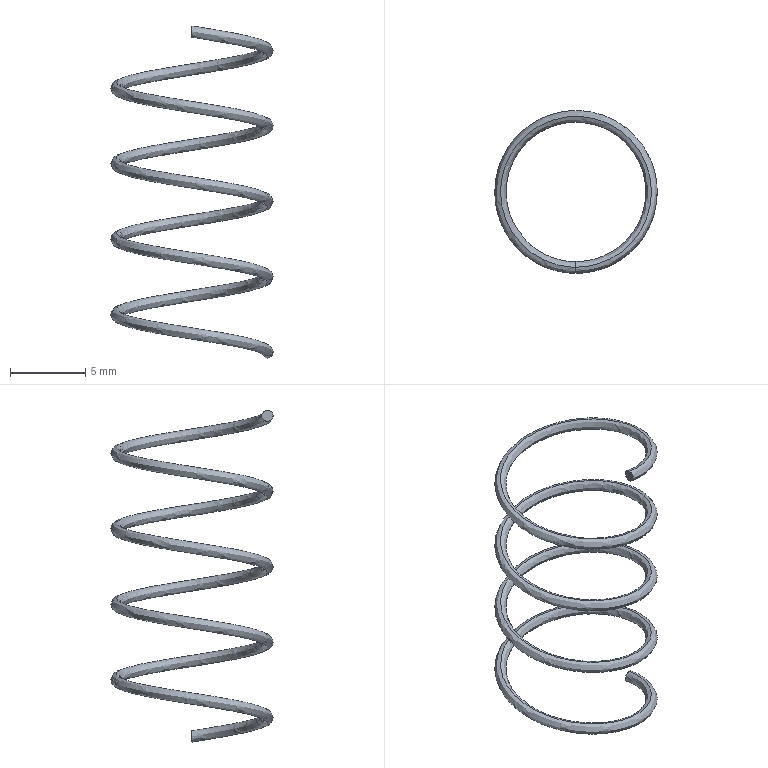Part | STEP file | Spring | 1 solid | 4 faces | box 10.75 x 10.75 x 22 mm | volume 58.932 mm3 | spline 2 | plane 2